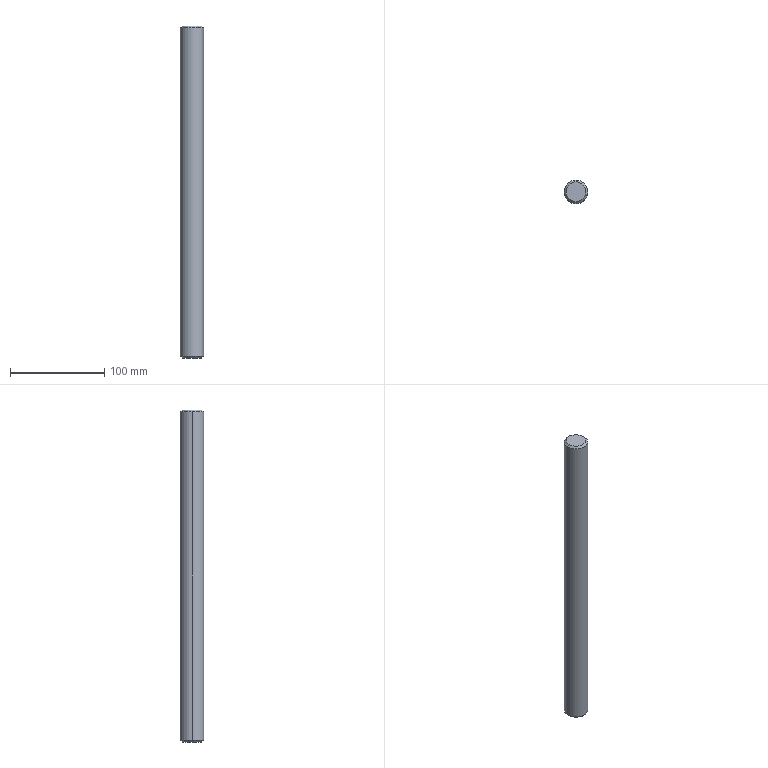Part | 1 solid | 8 faces | box 25 x 25 x 353 mm | volume 172981 mm3 | cone 4 | cylinder 2 | plane 2 | commonest cylinder face diameters 25 x2
STEP:
#1=CARTESIAN_POINT('',(10.5,0.,176.5));
#2=VERTEX_POINT('',#1);
#3=CARTESIAN_POINT('',(-10.5,0.,176.5));
#4=VERTEX_POINT('',#3);
#5=CARTESIAN_POINT('',(0.,0.,176.5));
#6=DIRECTION('',(0.,0.,1.));
#7=DIRECTION('',(1.,0.,0.));
#8=AXIS2_PLACEMENT_3D('',#5,#6,#7);
#9=CIRCLE('',#8,10.5);
#10=EDGE_CURVE('',#2,#4,#9,.T.);
#11=ORIENTED_EDGE('',*,*,#10,.F.);
#12=CARTESIAN_POINT('',(12.5,0.,174.5));
#13=VERTEX_POINT('',#12);
#14=CARTESIAN_POINT('',(10.5,0.,176.5));
#15=DIRECTION('',(0.7071,0.,-0.7071));
#16=VECTOR('',#15,1000.);
#17=LINE('',#14,#16);
#18=EDGE_CURVE('',#2,#13,#17,.T.);
#19=ORIENTED_EDGE('',*,*,#18,.T.);
#20=CARTESIAN_POINT('',(-12.5,0.,174.5));
#21=VERTEX_POINT('',#20);
#22=CARTESIAN_POINT('',(0.,0.,174.5));
#23=DIRECTION('',(0.,0.,1.));
#24=DIRECTION('',(1.,0.,0.));
#25=AXIS2_PLACEMENT_3D('',#22,#23,#24);
#26=CIRCLE('',#25,12.5);
#27=EDGE_CURVE('',#13,#21,#26,.T.);
#28=ORIENTED_EDGE('',*,*,#27,.T.);
#29=CARTESIAN_POINT('',(-10.5,0.,176.5));
#30=DIRECTION('',(-0.7071,0.,-0.7071));
#31=VECTOR('',#30,1000.);
#32=LINE('',#29,#31);
#33=EDGE_CURVE('',#4,#21,#32,.T.);
#34=ORIENTED_EDGE('',*,*,#33,.F.);
#35=EDGE_LOOP('',(#11,#19,#28,#34));
#36=FACE_OUTER_BOUND('',#35,.T.);
#37=CARTESIAN_POINT('',(0.,0.,176.5));
#38=DIRECTION('',(0.,0.,-1.));
#39=DIRECTION('',(-1.,0.,0.));
#40=AXIS2_PLACEMENT_3D('',#37,#38,#39);
#41=CONICAL_SURFACE('',#40,10.5,0.7854);
#42=ADVANCED_FACE('',(#36),#41,.T.);
#43=CARTESIAN_POINT('',(12.5,0.,-174.5));
#44=VERTEX_POINT('',#43);
#45=CARTESIAN_POINT('',(-12.5,0.,-174.5));
#46=VERTEX_POINT('',#45);
#47=CARTESIAN_POINT('',(0.,0.,-174.5));
#48=DIRECTION('',(0.,0.,1.));
#49=DIRECTION('',(1.,0.,0.));
#50=AXIS2_PLACEMENT_3D('',#47,#48,#49);
#51=CIRCLE('',#50,12.5);
#52=EDGE_CURVE('',#44,#46,#51,.T.);
#53=ORIENTED_EDGE('',*,*,#52,.T.);
#54=CARTESIAN_POINT('',(-12.5,0.,-176.5));
#55=DIRECTION('',(0.,0.,1.));
#56=VECTOR('',#55,1000.);
#57=LINE('',#54,#56);
#58=EDGE_CURVE('',#46,#21,#57,.T.);
#59=ORIENTED_EDGE('',*,*,#58,.T.);
#60=ORIENTED_EDGE('',*,*,#27,.F.);
#61=CARTESIAN_POINT('',(12.5,0.,-176.5));
#62=DIRECTION('',(0.,0.,1.));
#63=VECTOR('',#62,1000.);
#64=LINE('',#61,#63);
#65=EDGE_CURVE('',#44,#13,#64,.T.);
#66=ORIENTED_EDGE('',*,*,#65,.F.);
#67=EDGE_LOOP('',(#53,#59,#60,#66));
#68=FACE_OUTER_BOUND('',#67,.T.);
#69=CARTESIAN_POINT('',(0.,0.,-176.5));
#70=DIRECTION('',(0.,0.,1.));
#71=DIRECTION('',(1.,0.,0.));
#72=AXIS2_PLACEMENT_3D('',#69,#70,#71);
#73=CYLINDRICAL_SURFACE('',#72,12.5);
#74=ADVANCED_FACE('',(#68),#73,.T.);
#75=CARTESIAN_POINT('',(10.5,0.,-176.5));
#76=VERTEX_POINT('',#75);
#77=CARTESIAN_POINT('',(-10.5,0.,-176.5));
#78=VERTEX_POINT('',#77);
#79=CARTESIAN_POINT('',(0.,0.,-176.5));
#80=DIRECTION('',(0.,0.,1.));
#81=DIRECTION('',(1.,0.,0.));
#82=AXIS2_PLACEMENT_3D('',#79,#80,#81);
#83=CIRCLE('',#82,10.5);
#84=EDGE_CURVE('',#76,#78,#83,.T.);
#85=ORIENTED_EDGE('',*,*,#84,.T.);
#86=CARTESIAN_POINT('',(-12.5,0.,-174.5));
#87=DIRECTION('',(-0.7071,0.,0.7071));
#88=VECTOR('',#87,1000.);
#89=LINE('',#86,#88);
#90=EDGE_CURVE('',#78,#46,#89,.T.);
#91=ORIENTED_EDGE('',*,*,#90,.T.);
#92=ORIENTED_EDGE('',*,*,#52,.F.);
#93=CARTESIAN_POINT('',(12.5,0.,-174.5));
#94=DIRECTION('',(0.7071,0.,0.7071));
#95=VECTOR('',#94,1000.);
#96=LINE('',#93,#95);
#97=EDGE_CURVE('',#76,#44,#96,.T.);
#98=ORIENTED_EDGE('',*,*,#97,.F.);
#99=EDGE_LOOP('',(#85,#91,#92,#98));
#100=FACE_OUTER_BOUND('',#99,.T.);
#101=CARTESIAN_POINT('',(0.,0.,-174.5));
#102=DIRECTION('',(0.,0.,1.));
#103=DIRECTION('',(1.,0.,0.));
#104=AXIS2_PLACEMENT_3D('',#101,#102,#103);
#105=CONICAL_SURFACE('',#104,12.5,0.7854);
#106=ADVANCED_FACE('',(#100),#105,.T.);
#107=ORIENTED_EDGE('',*,*,#90,.F.);
#108=CARTESIAN_POINT('',(0.,0.,-176.5));
#109=DIRECTION('',(0.,0.,1.));
#110=DIRECTION('',(1.,0.,0.));
#111=AXIS2_PLACEMENT_3D('',#108,#109,#110);
#112=CIRCLE('',#111,10.5);
#113=EDGE_CURVE('',#78,#76,#112,.T.);
#114=ORIENTED_EDGE('',*,*,#113,.T.);
#115=ORIENTED_EDGE('',*,*,#97,.T.);
#116=CARTESIAN_POINT('',(0.,0.,-174.5));
#117=DIRECTION('',(0.,0.,1.));
#118=DIRECTION('',(1.,0.,0.));
#119=AXIS2_PLACEMENT_3D('',#116,#117,#118);
#120=CIRCLE('',#119,12.5);
#121=EDGE_CURVE('',#46,#44,#120,.T.);
#122=ORIENTED_EDGE('',*,*,#121,.F.);
#123=EDGE_LOOP('',(#107,#114,#115,#122));
#124=FACE_OUTER_BOUND('',#123,.T.);
#125=CARTESIAN_POINT('',(0.,0.,-174.5));
#126=DIRECTION('',(0.,0.,1.));
#127=DIRECTION('',(1.,0.,0.));
#128=AXIS2_PLACEMENT_3D('',#125,#126,#127);
#129=CONICAL_SURFACE('',#128,12.5,0.7854);
#130=ADVANCED_FACE('',(#124),#129,.T.);
#131=ORIENTED_EDGE('',*,*,#58,.F.);
#132=ORIENTED_EDGE('',*,*,#121,.T.);
#133=ORIENTED_EDGE('',*,*,#65,.T.);
#134=CARTESIAN_POINT('',(0.,0.,174.5));
#135=DIRECTION('',(0.,0.,1.));
#136=DIRECTION('',(1.,0.,0.));
#137=AXIS2_PLACEMENT_3D('',#134,#135,#136);
#138=CIRCLE('',#137,12.5);
#139=EDGE_CURVE('',#21,#13,#138,.T.);
#140=ORIENTED_EDGE('',*,*,#139,.F.);
#141=EDGE_LOOP('',(#131,#132,#133,#140));
#142=FACE_OUTER_BOUND('',#141,.T.);
#143=CARTESIAN_POINT('',(0.,0.,-176.5));
#144=DIRECTION('',(0.,0.,1.));
#145=DIRECTION('',(1.,0.,0.));
#146=AXIS2_PLACEMENT_3D('',#143,#144,#145);
#147=CYLINDRICAL_SURFACE('',#146,12.5);
#148=ADVANCED_FACE('',(#142),#147,.T.);
#149=ORIENTED_EDGE('',*,*,#18,.F.);
#150=CARTESIAN_POINT('',(0.,0.,176.5));
#151=DIRECTION('',(0.,0.,1.));
#152=DIRECTION('',(1.,0.,0.));
#153=AXIS2_PLACEMENT_3D('',#150,#151,#152);
#154=CIRCLE('',#153,10.5);
#155=EDGE_CURVE('',#4,#2,#154,.T.);
#156=ORIENTED_EDGE('',*,*,#155,.F.);
#157=ORIENTED_EDGE('',*,*,#33,.T.);
#158=ORIENTED_EDGE('',*,*,#139,.T.);
#159=EDGE_LOOP('',(#149,#156,#157,#158));
#160=FACE_OUTER_BOUND('',#159,.T.);
#161=CARTESIAN_POINT('',(0.,0.,176.5));
#162=DIRECTION('',(0.,0.,-1.));
#163=DIRECTION('',(-1.,0.,0.));
#164=AXIS2_PLACEMENT_3D('',#161,#162,#163);
#165=CONICAL_SURFACE('',#164,10.5,0.7854);
#166=ADVANCED_FACE('',(#160),#165,.T.);
#167=ORIENTED_EDGE('',*,*,#155,.T.);
#168=ORIENTED_EDGE('',*,*,#10,.T.);
#169=EDGE_LOOP('',(#167,#168));
#170=FACE_OUTER_BOUND('',#169,.T.);
#171=CARTESIAN_POINT('',(0.,0.,176.5));
#172=DIRECTION('',(0.,0.,1.));
#173=DIRECTION('',(1.,0.,0.));
#174=AXIS2_PLACEMENT_3D('',#171,#172,#173);
#175=PLANE('',#174);
#176=ADVANCED_FACE('',(#170),#175,.T.);
#177=ORIENTED_EDGE('',*,*,#84,.F.);
#178=ORIENTED_EDGE('',*,*,#113,.F.);
#179=EDGE_LOOP('',(#177,#178));
#180=FACE_OUTER_BOUND('',#179,.T.);
#181=CARTESIAN_POINT('',(10.5,0.,-176.5));
#182=DIRECTION('',(0.,0.,-1.));
#183=DIRECTION('',(-1.,0.,0.));
#184=AXIS2_PLACEMENT_3D('',#181,#182,#183);
#185=PLANE('',#184);
#186=ADVANCED_FACE('',(#180),#185,.T.);
#187=CLOSED_SHELL('',(#42,#74,#106,#130,#148,#166,#176,#186));
#188=MANIFOLD_SOLID_BREP('',#187);
#189=CARTESIAN_POINT('',(0.,0.,0.));
#190=DIRECTION('',(0.,0.,1.));
#191=DIRECTION('',(1.,0.,0.));
#192=AXIS2_PLACEMENT_3D('',#189,#190,#191);
#193=(LENGTH_UNIT()NAMED_UNIT(*)SI_UNIT(.MILLI.,.METRE.));
#194=UNCERTAINTY_MEASURE_WITH_UNIT(LENGTH_MEASURE(0.00001),#193,'','');
#195=(NAMED_UNIT(*)PLANE_ANGLE_UNIT()SI_UNIT($,.RADIAN.));
#196=(NAMED_UNIT(*)SI_UNIT($,.STERADIAN.)SOLID_ANGLE_UNIT());
#197=(GEOMETRIC_REPRESENTATION_CONTEXT(3)GLOBAL_UNCERTAINTY_ASSIGNED_CONTEXT((#194))GLOBAL_UNIT_ASSIGNED_CONTEXT((#193,#195,#196))REPRESENTATION_CONTEXT('',''));
#198=ADVANCED_BREP_SHAPE_REPRESENTATION('',(#188,#192),#197);